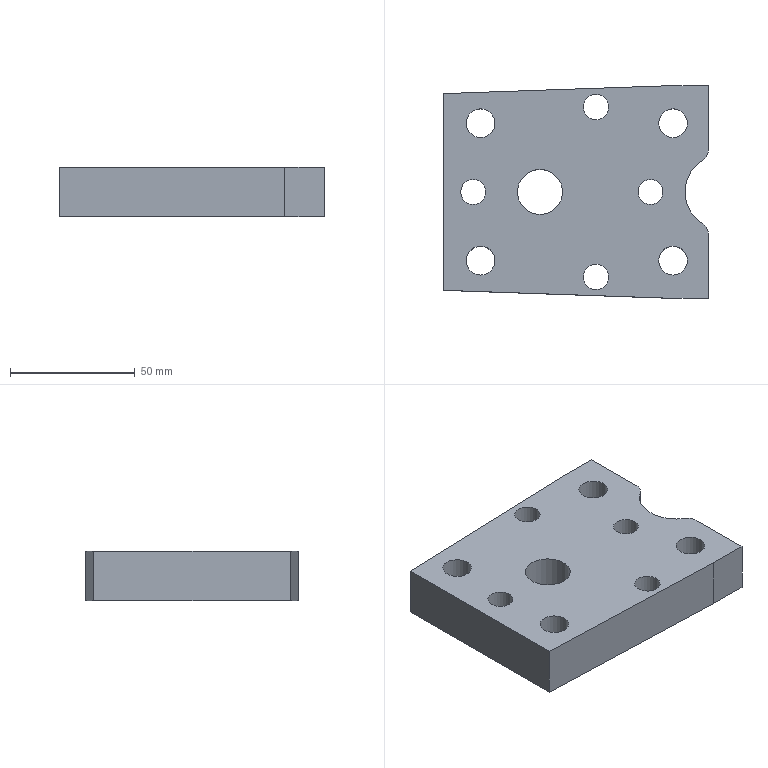Part | NX | features LB-13 2 | 1 solid | 21 faces | box 106 x 85 x 20 mm | volume 150874 mm3 | cylinder 12 | plane 9 | commonest cylinder face diameters 10 x4 11.5 x4 10.201 x2 18.003 x1 30.003 x1
STEP:
#1=CARTESIAN_POINT('',(3745.094,-818.769,803.716));
#2=VERTEX_POINT('',#1);
#3=CARTESIAN_POINT('',(3745.094,-818.769,823.716));
#4=VERTEX_POINT('',#3);
#5=CARTESIAN_POINT('',(3745.094,-818.769,858.716));
#6=DIRECTION('',(0.,0.,1.));
#7=VECTOR('',#6,1000.);
#8=LINE('',#5,#7);
#9=EDGE_CURVE('',#2,#4,#8,.T.);
#10=ORIENTED_EDGE('',*,*,#9,.F.);
#11=CARTESIAN_POINT('',(3745.094,-897.476,803.716));
#12=VERTEX_POINT('',#11);
#13=CARTESIAN_POINT('',(3745.094,-839.123,803.716));
#14=DIRECTION('',(0.,-1.,0.000000114));
#15=VECTOR('',#14,1000.);
#16=LINE('',#13,#15);
#17=EDGE_CURVE('',#12,#2,#16,.F.);
#18=ORIENTED_EDGE('',*,*,#17,.F.);
#19=CARTESIAN_POINT('',(3745.094,-897.476,823.716));
#20=VERTEX_POINT('',#19);
#21=CARTESIAN_POINT('',(3745.094,-897.476,858.716));
#22=DIRECTION('',(0.,0.,-1.));
#23=VECTOR('',#22,1000.);
#24=LINE('',#21,#23);
#25=EDGE_CURVE('',#20,#12,#24,.T.);
#26=ORIENTED_EDGE('',*,*,#25,.F.);
#27=CARTESIAN_POINT('',(3745.094,-839.123,823.716));
#28=DIRECTION('',(0.,-1.,0.000000114));
#29=VECTOR('',#28,1000.);
#30=LINE('',#27,#29);
#31=EDGE_CURVE('',#20,#4,#30,.F.);
#32=ORIENTED_EDGE('',*,*,#31,.T.);
#33=EDGE_LOOP('',(#10,#18,#26,#32));
#34=FACE_BOUND('',#33,.T.);
#35=CARTESIAN_POINT('',(3745.094,-999.122,858.716));
#36=DIRECTION('',(1.,0.,0.));
#37=DIRECTION('',(0.,0.,-1.));
#38=AXIS2_PLACEMENT_3D('',#35,#36,#37);
#39=PLANE('',#38);
#40=ADVANCED_FACE('',(#34),#39,.F.);
#41=CARTESIAN_POINT('',(3756.919,-853.122,823.716));
#42=VERTEX_POINT('',#41);
#43=CARTESIAN_POINT('',(3756.919,-858.122,823.716));
#44=DIRECTION('',(0.,-0.000000114,-1.));
#45=DIRECTION('',(0.,1.,-0.000000114));
#46=AXIS2_PLACEMENT_3D('',#43,#44,#45);
#47=CIRCLE('',#46,5.);
#48=EDGE_CURVE('',#42,#42,#47,.T.);
#49=ORIENTED_EDGE('',*,*,#48,.T.);
#50=EDGE_LOOP('',(#49));
#51=FACE_BOUND('',#50,.T.);
#52=CARTESIAN_POINT('',(3827.919,-853.122,823.716));
#53=VERTEX_POINT('',#52);
#54=CARTESIAN_POINT('',(3827.919,-858.122,823.716));
#55=DIRECTION('',(0.,-0.000000114,-1.));
#56=DIRECTION('',(0.,1.,-0.000000114));
#57=AXIS2_PLACEMENT_3D('',#54,#55,#56);
#58=CIRCLE('',#57,5.);
#59=EDGE_CURVE('',#53,#53,#58,.T.);
#60=ORIENTED_EDGE('',*,*,#59,.T.);
#61=EDGE_LOOP('',(#60));
#62=FACE_BOUND('',#61,.T.);
#63=CARTESIAN_POINT('',(3836.919,-824.872,823.716));
#64=VERTEX_POINT('',#63);
#65=CARTESIAN_POINT('',(3836.919,-830.622,823.716));
#66=DIRECTION('',(0.,-0.000000114,-1.));
#67=DIRECTION('',(0.,1.,-0.000000114));
#68=AXIS2_PLACEMENT_3D('',#65,#66,#67);
#69=CIRCLE('',#68,5.75);
#70=EDGE_CURVE('',#64,#64,#69,.T.);
#71=ORIENTED_EDGE('',*,*,#70,.T.);
#72=EDGE_LOOP('',(#71));
#73=FACE_BOUND('',#72,.T.);
#74=CARTESIAN_POINT('',(3759.919,-824.872,823.716));
#75=VERTEX_POINT('',#74);
#76=CARTESIAN_POINT('',(3759.919,-830.622,823.716));
#77=DIRECTION('',(0.,-0.000000114,-1.));
#78=DIRECTION('',(0.,1.,-0.000000114));
#79=AXIS2_PLACEMENT_3D('',#76,#77,#78);
#80=CIRCLE('',#79,5.75);
#81=EDGE_CURVE('',#75,#75,#80,.T.);
#82=ORIENTED_EDGE('',*,*,#81,.T.);
#83=EDGE_LOOP('',(#82));
#84=FACE_BOUND('',#83,.T.);
#85=CARTESIAN_POINT('',(3759.919,-879.872,823.716));
#86=VERTEX_POINT('',#85);
#87=CARTESIAN_POINT('',(3759.919,-885.622,823.716));
#88=DIRECTION('',(0.,-0.000000114,-1.));
#89=DIRECTION('',(0.,1.,-0.000000114));
#90=AXIS2_PLACEMENT_3D('',#87,#88,#89);
#91=CIRCLE('',#90,5.75);
#92=EDGE_CURVE('',#86,#86,#91,.T.);
#93=ORIENTED_EDGE('',*,*,#92,.T.);
#94=EDGE_LOOP('',(#93));
#95=FACE_BOUND('',#94,.T.);
#96=CARTESIAN_POINT('',(3836.919,-879.872,823.716));
#97=VERTEX_POINT('',#96);
#98=CARTESIAN_POINT('',(3836.919,-885.622,823.716));
#99=DIRECTION('',(0.,-0.000000114,-1.));
#100=DIRECTION('',(0.,1.,-0.000000114));
#101=AXIS2_PLACEMENT_3D('',#98,#99,#100);
#102=CIRCLE('',#101,5.75);
#103=EDGE_CURVE('',#97,#97,#102,.T.);
#104=ORIENTED_EDGE('',*,*,#103,.T.);
#105=EDGE_LOOP('',(#104));
#106=FACE_BOUND('',#105,.T.);
#107=CARTESIAN_POINT('',(3806.088,-819.043,823.716));
#108=VERTEX_POINT('',#107);
#109=CARTESIAN_POINT('',(3806.088,-824.144,823.716));
#110=DIRECTION('',(0.,-0.000000114,-1.));
#111=DIRECTION('',(0.,1.,-0.000000114));
#112=AXIS2_PLACEMENT_3D('',#109,#110,#111);
#113=CIRCLE('',#112,5.101);
#114=EDGE_CURVE('',#108,#108,#113,.F.);
#115=ORIENTED_EDGE('',*,*,#114,.F.);
#116=EDGE_LOOP('',(#115));
#117=FACE_BOUND('',#116,.T.);
#118=CARTESIAN_POINT('',(3783.699,-849.121,823.716));
#119=VERTEX_POINT('',#118);
#120=CARTESIAN_POINT('',(3783.699,-858.122,823.716));
#121=DIRECTION('',(0.,-0.000000114,-1.));
#122=DIRECTION('',(0.,1.,-0.000000114));
#123=AXIS2_PLACEMENT_3D('',#120,#121,#122);
#124=CIRCLE('',#123,9.002);
#125=EDGE_CURVE('',#119,#119,#124,.F.);
#126=ORIENTED_EDGE('',*,*,#125,.F.);
#127=EDGE_LOOP('',(#126));
#128=FACE_BOUND('',#127,.T.);
#129=CARTESIAN_POINT('',(3806.088,-887.001,823.716));
#130=VERTEX_POINT('',#129);
#131=CARTESIAN_POINT('',(3806.088,-892.101,823.716));
#132=DIRECTION('',(0.,-0.000000114,-1.));
#133=DIRECTION('',(0.,1.,-0.000000114));
#134=AXIS2_PLACEMENT_3D('',#131,#132,#133);
#135=CIRCLE('',#134,5.101);
#136=EDGE_CURVE('',#130,#130,#135,.T.);
#137=ORIENTED_EDGE('',*,*,#136,.T.);
#138=EDGE_LOOP('',(#137));
#139=FACE_BOUND('',#138,.T.);
#140=CARTESIAN_POINT('',(3835.207,-815.622,823.716));
#141=VERTEX_POINT('',#140);
#142=CARTESIAN_POINT('',(3979.71,-810.577,823.716));
#143=DIRECTION('',(0.9994,0.0349,-0.000000004));
#144=VECTOR('',#143,1000.);
#145=LINE('',#142,#144);
#146=EDGE_CURVE('',#4,#141,#145,.T.);
#147=ORIENTED_EDGE('',*,*,#146,.F.);
#148=ORIENTED_EDGE('',*,*,#31,.F.);
#149=CARTESIAN_POINT('',(3835.207,-900.622,823.716));
#150=VERTEX_POINT('',#149);
#151=CARTESIAN_POINT('',(3978.385,-905.622,823.716));
#152=DIRECTION('',(-0.9994,0.0349,-0.000000004));
#153=VECTOR('',#152,1000.);
#154=LINE('',#151,#153);
#155=EDGE_CURVE('',#150,#20,#154,.T.);
#156=ORIENTED_EDGE('',*,*,#155,.F.);
#157=CARTESIAN_POINT('',(3851.094,-900.622,823.716));
#158=VERTEX_POINT('',#157);
#159=CARTESIAN_POINT('',(3856.699,-900.622,823.716));
#160=DIRECTION('',(-1.,0.,0.));
#161=VECTOR('',#160,1000.);
#162=LINE('',#159,#161);
#163=EDGE_CURVE('',#158,#150,#162,.T.);
#164=ORIENTED_EDGE('',*,*,#163,.F.);
#165=CARTESIAN_POINT('',(3851.094,-875.081,823.716));
#166=VERTEX_POINT('',#165);
#167=CARTESIAN_POINT('',(3851.094,-839.123,823.716));
#168=DIRECTION('',(0.,1.,-0.000000114));
#169=VECTOR('',#168,1000.);
#170=LINE('',#167,#169);
#171=EDGE_CURVE('',#158,#166,#170,.T.);
#172=ORIENTED_EDGE('',*,*,#171,.T.);
#173=CARTESIAN_POINT('',(3848.745,-870.842,823.716));
#174=VERTEX_POINT('',#173);
#175=CARTESIAN_POINT('',(3846.094,-875.081,823.716));
#176=DIRECTION('',(0.,-0.000000114,-1.));
#177=DIRECTION('',(0.,1.,-0.000000114));
#178=AXIS2_PLACEMENT_3D('',#175,#176,#177);
#179=CIRCLE('',#178,5.);
#180=EDGE_CURVE('',#166,#174,#179,.F.);
#181=ORIENTED_EDGE('',*,*,#180,.T.);
#182=CARTESIAN_POINT('',(3848.745,-845.403,823.716));
#183=VERTEX_POINT('',#182);
#184=CARTESIAN_POINT('',(3856.699,-858.122,823.716));
#185=DIRECTION('',(0.,-0.000000114,-1.));
#186=DIRECTION('',(0.,1.,-0.000000114));
#187=AXIS2_PLACEMENT_3D('',#184,#185,#186);
#188=CIRCLE('',#187,15.002);
#189=EDGE_CURVE('',#183,#174,#188,.F.);
#190=ORIENTED_EDGE('',*,*,#189,.F.);
#191=CARTESIAN_POINT('',(3851.094,-841.164,823.716));
#192=VERTEX_POINT('',#191);
#193=CARTESIAN_POINT('',(3846.094,-841.164,823.716));
#194=DIRECTION('',(0.,-0.000000114,-1.));
#195=DIRECTION('',(0.,1.,-0.000000114));
#196=AXIS2_PLACEMENT_3D('',#193,#194,#195);
#197=CIRCLE('',#196,5.);
#198=EDGE_CURVE('',#183,#192,#197,.F.);
#199=ORIENTED_EDGE('',*,*,#198,.T.);
#200=CARTESIAN_POINT('',(3851.094,-815.622,823.716));
#201=VERTEX_POINT('',#200);
#202=CARTESIAN_POINT('',(3851.094,-839.123,823.716));
#203=DIRECTION('',(0.,1.,-0.000000114));
#204=VECTOR('',#203,1000.);
#205=LINE('',#202,#204);
#206=EDGE_CURVE('',#192,#201,#205,.T.);
#207=ORIENTED_EDGE('',*,*,#206,.T.);
#208=CARTESIAN_POINT('',(3856.699,-815.622,823.716));
#209=DIRECTION('',(-1.,0.,0.));
#210=VECTOR('',#209,1000.);
#211=LINE('',#208,#210);
#212=EDGE_CURVE('',#141,#201,#211,.F.);
#213=ORIENTED_EDGE('',*,*,#212,.F.);
#214=EDGE_LOOP('',(#147,#148,#156,#164,#172,#181,#190,#199,#207,#213));
#215=FACE_BOUND('',#214,.T.);
#216=CARTESIAN_POINT('',(3980.707,-839.123,823.716));
#217=DIRECTION('',(0.,-0.000000114,-1.));
#218=DIRECTION('',(0.,-1.,0.000000114));
#219=AXIS2_PLACEMENT_3D('',#216,#217,#218);
#220=PLANE('',#219);
#221=ADVANCED_FACE('',(#51,#62,#73,#84,#95,#106,#117,#128,#139,#215),#220,.F.);
#222=CARTESIAN_POINT('',(3756.919,-853.122,803.716));
#223=VERTEX_POINT('',#222);
#224=CARTESIAN_POINT('',(3756.919,-858.122,803.716));
#225=DIRECTION('',(0.,-0.000000114,-1.));
#226=DIRECTION('',(0.,1.,-0.000000114));
#227=AXIS2_PLACEMENT_3D('',#224,#225,#226);
#228=CIRCLE('',#227,5.);
#229=EDGE_CURVE('',#223,#223,#228,.F.);
#230=ORIENTED_EDGE('',*,*,#229,.T.);
#231=EDGE_LOOP('',(#230));
#232=FACE_BOUND('',#231,.T.);
#233=CARTESIAN_POINT('',(3827.919,-853.122,803.716));
#234=VERTEX_POINT('',#233);
#235=CARTESIAN_POINT('',(3827.919,-858.122,803.716));
#236=DIRECTION('',(0.,-0.000000114,-1.));
#237=DIRECTION('',(0.,1.,-0.000000114));
#238=AXIS2_PLACEMENT_3D('',#235,#236,#237);
#239=CIRCLE('',#238,5.);
#240=EDGE_CURVE('',#234,#234,#239,.F.);
#241=ORIENTED_EDGE('',*,*,#240,.T.);
#242=EDGE_LOOP('',(#241));
#243=FACE_BOUND('',#242,.T.);
#244=CARTESIAN_POINT('',(3836.919,-824.872,803.716));
#245=VERTEX_POINT('',#244);
#246=CARTESIAN_POINT('',(3836.919,-830.622,803.716));
#247=DIRECTION('',(0.,-0.000000114,-1.));
#248=DIRECTION('',(0.,1.,-0.000000114));
#249=AXIS2_PLACEMENT_3D('',#246,#247,#248);
#250=CIRCLE('',#249,5.75);
#251=EDGE_CURVE('',#245,#245,#250,.F.);
#252=ORIENTED_EDGE('',*,*,#251,.T.);
#253=EDGE_LOOP('',(#252));
#254=FACE_BOUND('',#253,.T.);
#255=CARTESIAN_POINT('',(3759.919,-824.872,803.716));
#256=VERTEX_POINT('',#255);
#257=CARTESIAN_POINT('',(3759.919,-830.622,803.716));
#258=DIRECTION('',(0.,-0.000000114,-1.));
#259=DIRECTION('',(0.,1.,-0.000000114));
#260=AXIS2_PLACEMENT_3D('',#257,#258,#259);
#261=CIRCLE('',#260,5.75);
#262=EDGE_CURVE('',#256,#256,#261,.F.);
#263=ORIENTED_EDGE('',*,*,#262,.T.);
#264=EDGE_LOOP('',(#263));
#265=FACE_BOUND('',#264,.T.);
#266=CARTESIAN_POINT('',(3759.919,-879.872,803.716));
#267=VERTEX_POINT('',#266);
#268=CARTESIAN_POINT('',(3759.919,-885.622,803.716));
#269=DIRECTION('',(0.,-0.000000114,-1.));
#270=DIRECTION('',(0.,1.,-0.000000114));
#271=AXIS2_PLACEMENT_3D('',#268,#269,#270);
#272=CIRCLE('',#271,5.75);
#273=EDGE_CURVE('',#267,#267,#272,.F.);
#274=ORIENTED_EDGE('',*,*,#273,.T.);
#275=EDGE_LOOP('',(#274));
#276=FACE_BOUND('',#275,.T.);
#277=CARTESIAN_POINT('',(3836.919,-879.872,803.716));
#278=VERTEX_POINT('',#277);
#279=CARTESIAN_POINT('',(3836.919,-885.622,803.716));
#280=DIRECTION('',(0.,-0.000000114,-1.));
#281=DIRECTION('',(0.,1.,-0.000000114));
#282=AXIS2_PLACEMENT_3D('',#279,#280,#281);
#283=CIRCLE('',#282,5.75);
#284=EDGE_CURVE('',#278,#278,#283,.F.);
#285=ORIENTED_EDGE('',*,*,#284,.T.);
#286=EDGE_LOOP('',(#285));
#287=FACE_BOUND('',#286,.T.);
#288=CARTESIAN_POINT('',(3783.699,-849.121,803.716));
#289=VERTEX_POINT('',#288);
#290=CARTESIAN_POINT('',(3783.699,-858.122,803.716));
#291=DIRECTION('',(0.,-0.000000114,-1.));
#292=DIRECTION('',(0.,1.,-0.000000114));
#293=AXIS2_PLACEMENT_3D('',#290,#291,#292);
#294=CIRCLE('',#293,9.002);
#295=EDGE_CURVE('',#289,#289,#294,.F.);
#296=ORIENTED_EDGE('',*,*,#295,.T.);
#297=EDGE_LOOP('',(#296));
#298=FACE_BOUND('',#297,.T.);
#299=CARTESIAN_POINT('',(3806.088,-887.001,803.716));
#300=VERTEX_POINT('',#299);
#301=CARTESIAN_POINT('',(3806.088,-892.101,803.716));
#302=DIRECTION('',(0.,-0.000000114,-1.));
#303=DIRECTION('',(0.,1.,-0.000000114));
#304=AXIS2_PLACEMENT_3D('',#301,#302,#303);
#305=CIRCLE('',#304,5.101);
#306=EDGE_CURVE('',#300,#300,#305,.T.);
#307=ORIENTED_EDGE('',*,*,#306,.F.);
#308=EDGE_LOOP('',(#307));
#309=FACE_BOUND('',#308,.T.);
#310=CARTESIAN_POINT('',(3806.088,-819.043,803.716));
#311=VERTEX_POINT('',#310);
#312=CARTESIAN_POINT('',(3806.088,-824.144,803.716));
#313=DIRECTION('',(0.,-0.000000114,-1.));
#314=DIRECTION('',(0.,1.,-0.000000114));
#315=AXIS2_PLACEMENT_3D('',#312,#313,#314);
#316=CIRCLE('',#315,5.101);
#317=EDGE_CURVE('',#311,#311,#316,.F.);
#318=ORIENTED_EDGE('',*,*,#317,.T.);
#319=EDGE_LOOP('',(#318));
#320=FACE_BOUND('',#319,.T.);
#321=ORIENTED_EDGE('',*,*,#17,.T.);
#322=CARTESIAN_POINT('',(3835.207,-815.622,803.716));
#323=VERTEX_POINT('',#322);
#324=CARTESIAN_POINT('',(3979.71,-810.577,803.716));
#325=DIRECTION('',(0.9994,0.0349,-0.000000004));
#326=VECTOR('',#325,1000.);
#327=LINE('',#324,#326);
#328=EDGE_CURVE('',#323,#2,#327,.F.);
#329=ORIENTED_EDGE('',*,*,#328,.F.);
#330=CARTESIAN_POINT('',(3851.094,-815.622,803.716));
#331=VERTEX_POINT('',#330);
#332=CARTESIAN_POINT('',(3856.699,-815.622,803.716));
#333=DIRECTION('',(-1.,0.,0.));
#334=VECTOR('',#333,1000.);
#335=LINE('',#332,#334);
#336=EDGE_CURVE('',#323,#331,#335,.F.);
#337=ORIENTED_EDGE('',*,*,#336,.T.);
#338=CARTESIAN_POINT('',(3851.094,-841.164,803.716));
#339=VERTEX_POINT('',#338);
#340=CARTESIAN_POINT('',(3851.094,-839.123,803.716));
#341=DIRECTION('',(0.,1.,-0.000000114));
#342=VECTOR('',#341,1000.);
#343=LINE('',#340,#342);
#344=EDGE_CURVE('',#339,#331,#343,.T.);
#345=ORIENTED_EDGE('',*,*,#344,.F.);
#346=CARTESIAN_POINT('',(3848.745,-845.403,803.716));
#347=VERTEX_POINT('',#346);
#348=CARTESIAN_POINT('',(3846.094,-841.164,803.716));
#349=DIRECTION('',(0.,-0.000000114,-1.));
#350=DIRECTION('',(0.,1.,-0.000000114));
#351=AXIS2_PLACEMENT_3D('',#348,#349,#350);
#352=CIRCLE('',#351,5.);
#353=EDGE_CURVE('',#339,#347,#352,.T.);
#354=ORIENTED_EDGE('',*,*,#353,.T.);
#355=CARTESIAN_POINT('',(3848.745,-870.842,803.716));
#356=VERTEX_POINT('',#355);
#357=CARTESIAN_POINT('',(3856.699,-858.122,803.716));
#358=DIRECTION('',(0.,-0.000000114,-1.));
#359=DIRECTION('',(0.,1.,-0.000000114));
#360=AXIS2_PLACEMENT_3D('',#357,#358,#359);
#361=CIRCLE('',#360,15.002);
#362=EDGE_CURVE('',#347,#356,#361,.F.);
#363=ORIENTED_EDGE('',*,*,#362,.T.);
#364=CARTESIAN_POINT('',(3851.094,-875.081,803.716));
#365=VERTEX_POINT('',#364);
#366=CARTESIAN_POINT('',(3846.094,-875.081,803.716));
#367=DIRECTION('',(0.,-0.000000114,-1.));
#368=DIRECTION('',(0.,1.,-0.000000114));
#369=AXIS2_PLACEMENT_3D('',#366,#367,#368);
#370=CIRCLE('',#369,5.);
#371=EDGE_CURVE('',#356,#365,#370,.T.);
#372=ORIENTED_EDGE('',*,*,#371,.T.);
#373=CARTESIAN_POINT('',(3851.094,-900.622,803.716));
#374=VERTEX_POINT('',#373);
#375=CARTESIAN_POINT('',(3851.094,-839.123,803.716));
#376=DIRECTION('',(0.,1.,-0.000000114));
#377=VECTOR('',#376,1000.);
#378=LINE('',#375,#377);
#379=EDGE_CURVE('',#374,#365,#378,.T.);
#380=ORIENTED_EDGE('',*,*,#379,.F.);
#381=CARTESIAN_POINT('',(3835.207,-900.622,803.716));
#382=VERTEX_POINT('',#381);
#383=CARTESIAN_POINT('',(3856.699,-900.622,803.716));
#384=DIRECTION('',(-1.,0.,0.));
#385=VECTOR('',#384,1000.);
#386=LINE('',#383,#385);
#387=EDGE_CURVE('',#374,#382,#386,.T.);
#388=ORIENTED_EDGE('',*,*,#387,.T.);
#389=CARTESIAN_POINT('',(3978.385,-905.622,803.716));
#390=DIRECTION('',(-0.9994,0.0349,-0.000000004));
#391=VECTOR('',#390,1000.);
#392=LINE('',#389,#391);
#393=EDGE_CURVE('',#12,#382,#392,.F.);
#394=ORIENTED_EDGE('',*,*,#393,.F.);
#395=EDGE_LOOP('',(#321,#329,#337,#345,#354,#363,#372,#380,#388,#394));
#396=FACE_BOUND('',#395,.T.);
#397=CARTESIAN_POINT('',(3980.707,-839.123,803.716));
#398=DIRECTION('',(0.,-0.000000114,-1.));
#399=DIRECTION('',(0.,-1.,0.000000114));
#400=AXIS2_PLACEMENT_3D('',#397,#398,#399);
#401=PLANE('',#400);
#402=ADVANCED_FACE('',(#232,#243,#254,#265,#276,#287,#298,#309,#320,#396),#401,.T.);
#403=ORIENTED_EDGE('',*,*,#336,.F.);
#404=CARTESIAN_POINT('',(3835.207,-815.622,858.716));
#405=DIRECTION('',(0.,0.,1.));
#406=VECTOR('',#405,1000.);
#407=LINE('',#404,#406);
#408=EDGE_CURVE('',#141,#323,#407,.F.);
#409=ORIENTED_EDGE('',*,*,#408,.F.);
#410=ORIENTED_EDGE('',*,*,#212,.T.);
#411=CARTESIAN_POINT('',(3851.094,-815.622,858.716));
#412=DIRECTION('',(0.,0.,1.));
#413=VECTOR('',#412,1000.);
#414=LINE('',#411,#413);
#415=EDGE_CURVE('',#331,#201,#414,.T.);
#416=ORIENTED_EDGE('',*,*,#415,.F.);
#417=EDGE_LOOP('',(#403,#409,#410,#416));
#418=FACE_BOUND('',#417,.T.);
#419=CARTESIAN_POINT('',(3856.699,-815.622,858.716));
#420=DIRECTION('',(0.,1.,0.));
#421=DIRECTION('',(0.,0.,1.));
#422=AXIS2_PLACEMENT_3D('',#419,#420,#421);
#423=PLANE('',#422);
#424=ADVANCED_FACE('',(#418),#423,.T.);
#425=ORIENTED_EDGE('',*,*,#163,.T.);
#426=CARTESIAN_POINT('',(3835.207,-900.622,858.716));
#427=DIRECTION('',(0.,0.,1.));
#428=VECTOR('',#427,1000.);
#429=LINE('',#426,#428);
#430=EDGE_CURVE('',#150,#382,#429,.F.);
#431=ORIENTED_EDGE('',*,*,#430,.T.);
#432=ORIENTED_EDGE('',*,*,#387,.F.);
#433=CARTESIAN_POINT('',(3851.094,-900.622,813.716));
#434=DIRECTION('',(0.,0.,-1.));
#435=VECTOR('',#434,1000.);
#436=LINE('',#433,#435);
#437=EDGE_CURVE('',#374,#158,#436,.F.);
#438=ORIENTED_EDGE('',*,*,#437,.T.);
#439=EDGE_LOOP('',(#425,#431,#432,#438));
#440=FACE_BOUND('',#439,.T.);
#441=CARTESIAN_POINT('',(3856.699,-900.622,858.716));
#442=DIRECTION('',(0.,1.,0.));
#443=DIRECTION('',(0.,0.,1.));
#444=AXIS2_PLACEMENT_3D('',#441,#442,#443);
#445=PLANE('',#444);
#446=ADVANCED_FACE('',(#440),#445,.F.);
#447=ORIENTED_EDGE('',*,*,#306,.T.);
#448=EDGE_LOOP('',(#447));
#449=FACE_BOUND('',#448,.T.);
#450=ORIENTED_EDGE('',*,*,#136,.F.);
#451=EDGE_LOOP('',(#450));
#452=FACE_BOUND('',#451,.T.);
#453=CARTESIAN_POINT('',(3806.088,-892.101,823.716));
#454=DIRECTION('',(0.,0.,-1.));
#455=DIRECTION('',(-1.,0.,0.));
#456=AXIS2_PLACEMENT_3D('',#453,#454,#455);
#457=CYLINDRICAL_SURFACE('',#456,5.101);
#458=ADVANCED_FACE('',(#449,#452),#457,.F.);
#459=ORIENTED_EDGE('',*,*,#125,.T.);
#460=EDGE_LOOP('',(#459));
#461=FACE_BOUND('',#460,.T.);
#462=ORIENTED_EDGE('',*,*,#295,.F.);
#463=EDGE_LOOP('',(#462));
#464=FACE_BOUND('',#463,.T.);
#465=CARTESIAN_POINT('',(3783.699,-858.122,802.716));
#466=DIRECTION('',(0.,0.,-1.));
#467=DIRECTION('',(1.,0.,0.));
#468=AXIS2_PLACEMENT_3D('',#465,#466,#467);
#469=CYLINDRICAL_SURFACE('',#468,9.002);
#470=ADVANCED_FACE('',(#461,#464),#469,.F.);
#471=ORIENTED_EDGE('',*,*,#317,.F.);
#472=EDGE_LOOP('',(#471));
#473=FACE_BOUND('',#472,.T.);
#474=ORIENTED_EDGE('',*,*,#114,.T.);
#475=EDGE_LOOP('',(#474));
#476=FACE_BOUND('',#475,.T.);
#477=CARTESIAN_POINT('',(3806.088,-824.144,823.716));
#478=DIRECTION('',(0.,0.,-1.));
#479=DIRECTION('',(-1.,0.,0.));
#480=AXIS2_PLACEMENT_3D('',#477,#478,#479);
#481=CYLINDRICAL_SURFACE('',#480,5.101);
#482=ADVANCED_FACE('',(#473,#476),#481,.F.);
#483=ORIENTED_EDGE('',*,*,#103,.F.);
#484=EDGE_LOOP('',(#483));
#485=FACE_BOUND('',#484,.T.);
#486=ORIENTED_EDGE('',*,*,#284,.F.);
#487=EDGE_LOOP('',(#486));
#488=FACE_BOUND('',#487,.T.);
#489=CARTESIAN_POINT('',(3836.919,-885.622,823.716));
#490=DIRECTION('',(0.,0.,-1.));
#491=DIRECTION('',(1.,0.,0.));
#492=AXIS2_PLACEMENT_3D('',#489,#490,#491);
#493=CYLINDRICAL_SURFACE('',#492,5.75);
#494=ADVANCED_FACE('',(#485,#488),#493,.F.);
#495=ORIENTED_EDGE('',*,*,#92,.F.);
#496=EDGE_LOOP('',(#495));
#497=FACE_BOUND('',#496,.T.);
#498=ORIENTED_EDGE('',*,*,#273,.F.);
#499=EDGE_LOOP('',(#498));
#500=FACE_BOUND('',#499,.T.);
#501=CARTESIAN_POINT('',(3759.919,-885.622,823.716));
#502=DIRECTION('',(0.,0.,-1.));
#503=DIRECTION('',(1.,0.,0.));
#504=AXIS2_PLACEMENT_3D('',#501,#502,#503);
#505=CYLINDRICAL_SURFACE('',#504,5.75);
#506=ADVANCED_FACE('',(#497,#500),#505,.F.);
#507=ORIENTED_EDGE('',*,*,#81,.F.);
#508=EDGE_LOOP('',(#507));
#509=FACE_BOUND('',#508,.T.);
#510=ORIENTED_EDGE('',*,*,#262,.F.);
#511=EDGE_LOOP('',(#510));
#512=FACE_BOUND('',#511,.T.);
#513=CARTESIAN_POINT('',(3759.919,-830.622,823.716));
#514=DIRECTION('',(0.,0.,-1.));
#515=DIRECTION('',(1.,0.,0.));
#516=AXIS2_PLACEMENT_3D('',#513,#514,#515);
#517=CYLINDRICAL_SURFACE('',#516,5.75);
#518=ADVANCED_FACE('',(#509,#512),#517,.F.);
#519=ORIENTED_EDGE('',*,*,#70,.F.);
#520=EDGE_LOOP('',(#519));
#521=FACE_BOUND('',#520,.T.);
#522=ORIENTED_EDGE('',*,*,#251,.F.);
#523=EDGE_LOOP('',(#522));
#524=FACE_BOUND('',#523,.T.);
#525=CARTESIAN_POINT('',(3836.919,-830.622,823.716));
#526=DIRECTION('',(0.,0.,-1.));
#527=DIRECTION('',(1.,0.,0.));
#528=AXIS2_PLACEMENT_3D('',#525,#526,#527);
#529=CYLINDRICAL_SURFACE('',#528,5.75);
#530=ADVANCED_FACE('',(#521,#524),#529,.F.);
#531=ORIENTED_EDGE('',*,*,#59,.F.);
#532=EDGE_LOOP('',(#531));
#533=FACE_BOUND('',#532,.T.);
#534=ORIENTED_EDGE('',*,*,#240,.F.);
#535=EDGE_LOOP('',(#534));
#536=FACE_BOUND('',#535,.T.);
#537=CARTESIAN_POINT('',(3827.919,-858.122,823.716));
#538=DIRECTION('',(0.,0.,-1.));
#539=DIRECTION('',(1.,0.,0.));
#540=AXIS2_PLACEMENT_3D('',#537,#538,#539);
#541=CYLINDRICAL_SURFACE('',#540,5.);
#542=ADVANCED_FACE('',(#533,#536),#541,.F.);
#543=ORIENTED_EDGE('',*,*,#48,.F.);
#544=EDGE_LOOP('',(#543));
#545=FACE_BOUND('',#544,.T.);
#546=ORIENTED_EDGE('',*,*,#229,.F.);
#547=EDGE_LOOP('',(#546));
#548=FACE_BOUND('',#547,.T.);
#549=CARTESIAN_POINT('',(3756.919,-858.122,823.716));
#550=DIRECTION('',(0.,0.,-1.));
#551=DIRECTION('',(1.,0.,0.));
#552=AXIS2_PLACEMENT_3D('',#549,#550,#551);
#553=CYLINDRICAL_SURFACE('',#552,5.);
#554=ADVANCED_FACE('',(#545,#548),#553,.F.);
#555=ORIENTED_EDGE('',*,*,#206,.F.);
#556=CARTESIAN_POINT('',(3851.094,-841.164,813.716));
#557=DIRECTION('',(0.,0.,-1.));
#558=VECTOR('',#557,1000.);
#559=LINE('',#556,#558);
#560=EDGE_CURVE('',#192,#339,#559,.T.);
#561=ORIENTED_EDGE('',*,*,#560,.T.);
#562=ORIENTED_EDGE('',*,*,#344,.T.);
#563=ORIENTED_EDGE('',*,*,#415,.T.);
#564=EDGE_LOOP('',(#555,#561,#562,#563));
#565=FACE_BOUND('',#564,.T.);
#566=CARTESIAN_POINT('',(3851.094,-904.872,813.716));
#567=DIRECTION('',(-1.,0.,0.));
#568=DIRECTION('',(0.,0.,1.));
#569=AXIS2_PLACEMENT_3D('',#566,#567,#568);
#570=PLANE('',#569);
#571=ADVANCED_FACE('',(#565),#570,.F.);
#572=ORIENTED_EDGE('',*,*,#379,.T.);
#573=CARTESIAN_POINT('',(3851.094,-875.081,813.716));
#574=DIRECTION('',(0.,0.,-1.));
#575=VECTOR('',#574,1000.);
#576=LINE('',#573,#575);
#577=EDGE_CURVE('',#365,#166,#576,.F.);
#578=ORIENTED_EDGE('',*,*,#577,.T.);
#579=ORIENTED_EDGE('',*,*,#171,.F.);
#580=ORIENTED_EDGE('',*,*,#437,.F.);
#581=EDGE_LOOP('',(#572,#578,#579,#580));
#582=FACE_BOUND('',#581,.T.);
#583=CARTESIAN_POINT('',(3851.094,-904.872,813.716));
#584=DIRECTION('',(-1.,0.,0.));
#585=DIRECTION('',(0.,0.,1.));
#586=AXIS2_PLACEMENT_3D('',#583,#584,#585);
#587=PLANE('',#586);
#588=ADVANCED_FACE('',(#582),#587,.F.);
#589=ORIENTED_EDGE('',*,*,#189,.T.);
#590=CARTESIAN_POINT('',(3848.745,-870.842,802.716));
#591=DIRECTION('',(0.,0.,-1.));
#592=VECTOR('',#591,1000.);
#593=LINE('',#590,#592);
#594=EDGE_CURVE('',#174,#356,#593,.T.);
#595=ORIENTED_EDGE('',*,*,#594,.T.);
#596=ORIENTED_EDGE('',*,*,#362,.F.);
#597=CARTESIAN_POINT('',(3848.745,-845.403,802.716));
#598=DIRECTION('',(0.,0.,-1.));
#599=VECTOR('',#598,1000.);
#600=LINE('',#597,#599);
#601=EDGE_CURVE('',#347,#183,#600,.F.);
#602=ORIENTED_EDGE('',*,*,#601,.T.);
#603=EDGE_LOOP('',(#589,#595,#596,#602));
#604=FACE_BOUND('',#603,.T.);
#605=CARTESIAN_POINT('',(3856.699,-858.122,802.716));
#606=DIRECTION('',(0.,0.,-1.));
#607=DIRECTION('',(1.,0.,0.));
#608=AXIS2_PLACEMENT_3D('',#605,#606,#607);
#609=CYLINDRICAL_SURFACE('',#608,15.002);
#610=ADVANCED_FACE('',(#604),#609,.F.);
#611=ORIENTED_EDGE('',*,*,#180,.F.);
#612=ORIENTED_EDGE('',*,*,#577,.F.);
#613=ORIENTED_EDGE('',*,*,#371,.F.);
#614=ORIENTED_EDGE('',*,*,#594,.F.);
#615=EDGE_LOOP('',(#611,#612,#613,#614));
#616=FACE_BOUND('',#615,.T.);
#617=CARTESIAN_POINT('',(3846.094,-875.081,802.716));
#618=DIRECTION('',(0.,0.,-1.));
#619=DIRECTION('',(-1.,0.,0.));
#620=AXIS2_PLACEMENT_3D('',#617,#618,#619);
#621=CYLINDRICAL_SURFACE('',#620,5.);
#622=ADVANCED_FACE('',(#616),#621,.T.);
#623=ORIENTED_EDGE('',*,*,#353,.F.);
#624=ORIENTED_EDGE('',*,*,#560,.F.);
#625=ORIENTED_EDGE('',*,*,#198,.F.);
#626=ORIENTED_EDGE('',*,*,#601,.F.);
#627=EDGE_LOOP('',(#623,#624,#625,#626));
#628=FACE_BOUND('',#627,.T.);
#629=CARTESIAN_POINT('',(3846.094,-841.164,802.716));
#630=DIRECTION('',(0.,0.,-1.));
#631=DIRECTION('',(-1.,0.,0.));
#632=AXIS2_PLACEMENT_3D('',#629,#630,#631);
#633=CYLINDRICAL_SURFACE('',#632,5.);
#634=ADVANCED_FACE('',(#628),#633,.T.);
#635=ORIENTED_EDGE('',*,*,#430,.F.);
#636=ORIENTED_EDGE('',*,*,#155,.T.);
#637=ORIENTED_EDGE('',*,*,#25,.T.);
#638=ORIENTED_EDGE('',*,*,#393,.T.);
#639=EDGE_LOOP('',(#635,#636,#637,#638));
#640=FACE_BOUND('',#639,.T.);
#641=CARTESIAN_POINT('',(3767.215,-898.248,841.216));
#642=DIRECTION('',(-0.0349,-0.9994,0.));
#643=DIRECTION('',(0.9994,-0.0349,0.));
#644=AXIS2_PLACEMENT_3D('',#641,#642,#643);
#645=PLANE('',#644);
#646=ADVANCED_FACE('',(#640),#645,.T.);
#647=ORIENTED_EDGE('',*,*,#328,.T.);
#648=ORIENTED_EDGE('',*,*,#9,.T.);
#649=ORIENTED_EDGE('',*,*,#146,.T.);
#650=ORIENTED_EDGE('',*,*,#408,.T.);
#651=EDGE_LOOP('',(#647,#648,#649,#650));
#652=FACE_BOUND('',#651,.T.);
#653=CARTESIAN_POINT('',(3767.215,-817.996,841.216));
#654=DIRECTION('',(-0.0349,0.9994,0.));
#655=DIRECTION('',(-0.9994,-0.0349,0.));
#656=AXIS2_PLACEMENT_3D('',#653,#654,#655);
#657=PLANE('',#656);
#658=ADVANCED_FACE('',(#652),#657,.T.);
#659=CLOSED_SHELL('',(#40,#221,#402,#424,#446,#458,#470,#482,#494,#506,#518,#530,#542,#554,#571,#588,#610,#622,#634,#646,#658));
#660=MANIFOLD_SOLID_BREP('',#659);
#661=(LENGTH_UNIT()NAMED_UNIT(*)SI_UNIT(.MILLI.,.METRE.));
#662=UNCERTAINTY_MEASURE_WITH_UNIT(LENGTH_MEASURE(0.00001),#661,'','');
#663=(NAMED_UNIT(*)PLANE_ANGLE_UNIT()SI_UNIT($,.RADIAN.));
#664=(NAMED_UNIT(*)SI_UNIT($,.STERADIAN.)SOLID_ANGLE_UNIT());
#665=(GEOMETRIC_REPRESENTATION_CONTEXT(3)GLOBAL_UNCERTAINTY_ASSIGNED_CONTEXT((#662))GLOBAL_UNIT_ASSIGNED_CONTEXT((#661,#663,#664))REPRESENTATION_CONTEXT('',''));
#666=ADVANCED_BREP_SHAPE_REPRESENTATION('',(#660),#665);